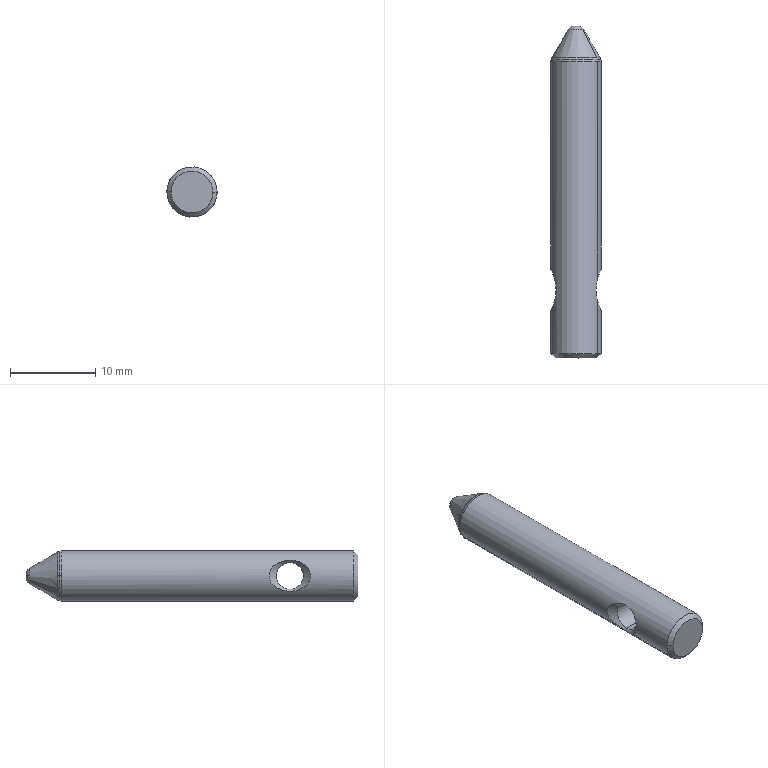Part | NX | features solid 2 | 1 solid | 20 faces | box 5.9 x 39 x 5.9 mm | volume 952.657 mm3 | cone 8 | cylinder 4 | torus 4 | plane 2 | spline 2 | commonest cylinder face diameters 3.2 x2 5.9 x2
STEP:
#1=CARTESIAN_POINT('',(-286.449,2108.126,25.582));
#2=VERTEX_POINT('',#1);
#3=CARTESIAN_POINT('',(-286.869,2108.126,27.147));
#4=VERTEX_POINT('',#3);
#5=CARTESIAN_POINT('',(-283.92,2108.126,27.1));
#6=DIRECTION('',(0.,1.,0.));
#7=DIRECTION('',(-0.8575,0.,-0.5144));
#8=AXIS2_PLACEMENT_3D('',#5,#6,#7);
#9=CIRCLE('',#8,2.95);
#10=EDGE_CURVE('',#2,#4,#9,.T.);
#11=ORIENTED_EDGE('',*,*,#10,.F.);
#12=CARTESIAN_POINT('',(-286.449,2082.541,25.582));
#13=VERTEX_POINT('',#12);
#14=CARTESIAN_POINT('',(-286.449,2108.126,25.582));
#15=DIRECTION('',(-0.000001242,-1.,0.00000207));
#16=VECTOR('',#15,1000.);
#17=LINE('',#14,#16);
#18=EDGE_CURVE('',#13,#2,#17,.F.);
#19=ORIENTED_EDGE('',*,*,#18,.F.);
#20=CARTESIAN_POINT('',(-286.211,2081.278,28.958));
#21=VERTEX_POINT('',#20);
#22=CARTESIAN_POINT('',(-286.211,2081.278,28.958));
#23=CARTESIAN_POINT('',(-286.211,2081.745,28.958));
#24=CARTESIAN_POINT('',(-286.382,2082.647,28.765));
#25=CARTESIAN_POINT('',(-286.775,2083.553,28.042));
#26=CARTESIAN_POINT('',(-286.9,2083.793,27.11));
#27=CARTESIAN_POINT('',(-286.784,2083.508,26.194));
#28=CARTESIAN_POINT('',(-286.562,2082.953,25.77));
#29=CARTESIAN_POINT('',(-286.449,2082.541,25.582));
#30=B_SPLINE_CURVE_WITH_KNOTS('',3,(#22,#23,#24,#25,#26,#27,#28,#29),.UNSPECIFIED.,.F.,.F.,(4,1,1,1,1,4),(0.,0.001381,0.002761,0.003452,0.004142,0.005523),.UNSPECIFIED.);
#31=EDGE_CURVE('',#21,#13,#30,.T.);
#32=ORIENTED_EDGE('',*,*,#31,.F.);
#33=CARTESIAN_POINT('',(-286.449,2080.015,25.582));
#34=VERTEX_POINT('',#33);
#35=CARTESIAN_POINT('',(-286.449,2080.015,25.582));
#36=CARTESIAN_POINT('',(-286.562,2079.603,25.77));
#37=CARTESIAN_POINT('',(-286.782,2079.051,26.189));
#38=CARTESIAN_POINT('',(-286.9,2078.763,27.107));
#39=CARTESIAN_POINT('',(-286.776,2079.,28.039));
#40=CARTESIAN_POINT('',(-286.384,2079.902,28.763));
#41=CARTESIAN_POINT('',(-286.211,2080.811,28.958));
#42=CARTESIAN_POINT('',(-286.211,2081.278,28.958));
#43=B_SPLINE_CURVE_WITH_KNOTS('',3,(#35,#36,#37,#38,#39,#40,#41,#42),.UNSPECIFIED.,.F.,.F.,(4,1,1,1,1,4),(0.,0.001379,0.002068,0.002758,0.004136,0.005515),.UNSPECIFIED.);
#44=EDGE_CURVE('',#34,#21,#43,.T.);
#45=ORIENTED_EDGE('',*,*,#44,.F.);
#46=CARTESIAN_POINT('',(-286.449,2073.778,25.582));
#47=VERTEX_POINT('',#46);
#48=CARTESIAN_POINT('',(-286.449,2080.015,25.582));
#49=DIRECTION('',(0.,-1.,0.));
#50=VECTOR('',#49,1000.);
#51=LINE('',#48,#50);
#52=EDGE_CURVE('',#47,#34,#51,.F.);
#53=ORIENTED_EDGE('',*,*,#52,.F.);
#54=CARTESIAN_POINT('',(-286.869,2073.778,27.147));
#55=VERTEX_POINT('',#54);
#56=CARTESIAN_POINT('',(-283.92,2073.778,27.1));
#57=DIRECTION('',(0.,-1.,0.));
#58=DIRECTION('',(-0.9999,0.,0.01589));
#59=AXIS2_PLACEMENT_3D('',#56,#57,#58);
#60=CIRCLE('',#59,2.95);
#61=EDGE_CURVE('',#55,#47,#60,.T.);
#62=ORIENTED_EDGE('',*,*,#61,.F.);
#63=CARTESIAN_POINT('',(-281.39,2073.778,28.618));
#64=VERTEX_POINT('',#63);
#65=CARTESIAN_POINT('',(-283.92,2073.778,27.1));
#66=DIRECTION('',(0.,-1.,0.));
#67=DIRECTION('',(0.8575,0.,0.5144));
#68=AXIS2_PLACEMENT_3D('',#65,#66,#67);
#69=CIRCLE('',#68,2.95);
#70=EDGE_CURVE('',#64,#55,#69,.T.);
#71=ORIENTED_EDGE('',*,*,#70,.F.);
#72=CARTESIAN_POINT('',(-281.39,2080.015,28.618));
#73=VERTEX_POINT('',#72);
#74=CARTESIAN_POINT('',(-281.39,2080.015,28.618));
#75=DIRECTION('',(0.,-1.,0.));
#76=VECTOR('',#75,1000.);
#77=LINE('',#74,#76);
#78=EDGE_CURVE('',#73,#64,#77,.T.);
#79=ORIENTED_EDGE('',*,*,#78,.F.);
#80=CARTESIAN_POINT('',(-281.57,2081.278,28.884));
#81=VERTEX_POINT('',#80);
#82=CARTESIAN_POINT('',(-281.57,2081.278,28.884));
#83=CARTESIAN_POINT('',(-281.57,2080.836,28.884));
#84=CARTESIAN_POINT('',(-281.496,2080.405,28.795));
#85=CARTESIAN_POINT('',(-281.39,2080.015,28.618));
#86=B_SPLINE_CURVE_WITH_KNOTS('',3,(#82,#83,#84,#85),.UNSPECIFIED.,.F.,.F.,(4,4),(0.,0.001307),.UNSPECIFIED.);
#87=EDGE_CURVE('',#81,#73,#86,.T.);
#88=ORIENTED_EDGE('',*,*,#87,.F.);
#89=CARTESIAN_POINT('',(-281.39,2082.541,28.618));
#90=VERTEX_POINT('',#89);
#91=CARTESIAN_POINT('',(-281.39,2082.541,28.618));
#92=CARTESIAN_POINT('',(-281.497,2082.15,28.795));
#93=CARTESIAN_POINT('',(-281.57,2081.72,28.884));
#94=CARTESIAN_POINT('',(-281.57,2081.278,28.884));
#95=B_SPLINE_CURVE_WITH_KNOTS('',3,(#91,#92,#93,#94),.UNSPECIFIED.,.F.,.F.,(4,4),(0.,0.001307),.UNSPECIFIED.);
#96=EDGE_CURVE('',#90,#81,#95,.T.);
#97=ORIENTED_EDGE('',*,*,#96,.F.);
#98=CARTESIAN_POINT('',(-281.39,2108.126,28.618));
#99=VERTEX_POINT('',#98);
#100=CARTESIAN_POINT('',(-281.39,2108.126,28.618));
#101=DIRECTION('',(0.,-1.,0.));
#102=VECTOR('',#101,1000.);
#103=LINE('',#100,#102);
#104=EDGE_CURVE('',#99,#90,#103,.T.);
#105=ORIENTED_EDGE('',*,*,#104,.F.);
#106=CARTESIAN_POINT('',(-283.92,2108.126,27.1));
#107=DIRECTION('',(0.,1.,0.));
#108=DIRECTION('',(-0.9999,0.,0.01589));
#109=AXIS2_PLACEMENT_3D('',#106,#107,#108);
#110=CIRCLE('',#109,2.95);
#111=EDGE_CURVE('',#4,#99,#110,.T.);
#112=ORIENTED_EDGE('',*,*,#111,.F.);
#113=EDGE_LOOP('',(#11,#19,#32,#45,#53,#62,#71,#79,#88,#97,#105,#112));
#114=FACE_BOUND('',#113,.T.);
#115=CARTESIAN_POINT('',(-283.92,2084.546,27.1));
#116=DIRECTION('',(0.,-1.,0.));
#117=DIRECTION('',(-0.8575,0.,-0.5144));
#118=AXIS2_PLACEMENT_3D('',#115,#116,#117);
#119=CYLINDRICAL_SURFACE('',#118,2.95);
#120=ADVANCED_FACE('',(#114),#119,.T.);
#121=CARTESIAN_POINT('',(-280.97,2108.126,27.053));
#122=VERTEX_POINT('',#121);
#123=CARTESIAN_POINT('',(-283.92,2108.126,27.1));
#124=DIRECTION('',(0.,1.,0.));
#125=DIRECTION('',(0.8575,0.,0.5144));
#126=AXIS2_PLACEMENT_3D('',#123,#124,#125);
#127=CIRCLE('',#126,2.95);
#128=EDGE_CURVE('',#99,#122,#127,.T.);
#129=ORIENTED_EDGE('',*,*,#128,.T.);
#130=CARTESIAN_POINT('',(-280.997,2108.333,27.054));
#131=VERTEX_POINT('',#130);
#132=CARTESIAN_POINT('',(-281.77,2108.126,27.066));
#133=DIRECTION('',(-0.01589,0.,-0.9999));
#134=DIRECTION('',(0.9658,0.2588,-0.01535));
#135=AXIS2_PLACEMENT_3D('',#132,#133,#134);
#136=CIRCLE('',#135,0.8);
#137=EDGE_CURVE('',#122,#131,#136,.F.);
#138=ORIENTED_EDGE('',*,*,#137,.T.);
#139=CARTESIAN_POINT('',(-286.842,2108.333,27.146));
#140=VERTEX_POINT('',#139);
#141=CARTESIAN_POINT('',(-283.92,2108.333,27.1));
#142=DIRECTION('',(0.,-1.,0.));
#143=DIRECTION('',(0.9999,0.,-0.01589));
#144=AXIS2_PLACEMENT_3D('',#141,#142,#143);
#145=CIRCLE('',#144,2.923);
#146=EDGE_CURVE('',#131,#140,#145,.T.);
#147=ORIENTED_EDGE('',*,*,#146,.T.);
#148=CARTESIAN_POINT('',(-286.069,2108.126,27.134));
#149=DIRECTION('',(0.01589,0.,0.9999));
#150=DIRECTION('',(-0.9658,0.2588,0.01535));
#151=AXIS2_PLACEMENT_3D('',#148,#149,#150);
#152=CIRCLE('',#151,0.8);
#153=EDGE_CURVE('',#140,#4,#152,.T.);
#154=ORIENTED_EDGE('',*,*,#153,.T.);
#155=ORIENTED_EDGE('',*,*,#111,.T.);
#156=EDGE_LOOP('',(#129,#138,#147,#154,#155));
#157=FACE_BOUND('',#156,.T.);
#158=CARTESIAN_POINT('',(-283.92,2108.126,27.1));
#159=DIRECTION('',(0.,-1.,0.));
#160=DIRECTION('',(-0.9999,0.,0.01589));
#161=AXIS2_PLACEMENT_3D('',#158,#159,#160);
#162=TOROIDAL_SURFACE('',#161,2.15,0.8);
#163=ADVANCED_FACE('',(#157),#162,.T.);
#164=ORIENTED_EDGE('',*,*,#153,.F.);
#165=CARTESIAN_POINT('',(-283.92,2108.333,27.1));
#166=DIRECTION('',(0.,-1.,0.));
#167=DIRECTION('',(-0.9999,0.,0.01589));
#168=AXIS2_PLACEMENT_3D('',#165,#166,#167);
#169=CIRCLE('',#168,2.923);
#170=EDGE_CURVE('',#140,#131,#169,.T.);
#171=ORIENTED_EDGE('',*,*,#170,.T.);
#172=ORIENTED_EDGE('',*,*,#137,.F.);
#173=CARTESIAN_POINT('',(-283.92,2108.126,27.1));
#174=DIRECTION('',(0.,1.,0.));
#175=DIRECTION('',(0.9999,0.,-0.01589));
#176=AXIS2_PLACEMENT_3D('',#173,#174,#175);
#177=CIRCLE('',#176,2.95);
#178=EDGE_CURVE('',#122,#2,#177,.T.);
#179=ORIENTED_EDGE('',*,*,#178,.T.);
#180=ORIENTED_EDGE('',*,*,#10,.T.);
#181=EDGE_LOOP('',(#164,#171,#172,#179,#180));
#182=FACE_BOUND('',#181,.T.);
#183=CARTESIAN_POINT('',(-283.92,2108.126,27.1));
#184=DIRECTION('',(0.,-1.,0.));
#185=DIRECTION('',(-0.9999,0.,0.01589));
#186=AXIS2_PLACEMENT_3D('',#183,#184,#185);
#187=TOROIDAL_SURFACE('',#186,2.15,0.8);
#188=ADVANCED_FACE('',(#182),#187,.T.);
#189=ORIENTED_EDGE('',*,*,#104,.T.);
#190=CARTESIAN_POINT('',(-281.628,2081.278,25.242));
#191=VERTEX_POINT('',#190);
#192=CARTESIAN_POINT('',(-281.628,2081.278,25.242));
#193=CARTESIAN_POINT('',(-281.628,2081.745,25.242));
#194=CARTESIAN_POINT('',(-281.457,2082.647,25.435));
#195=CARTESIAN_POINT('',(-281.065,2083.553,26.158));
#196=CARTESIAN_POINT('',(-280.94,2083.793,27.09));
#197=CARTESIAN_POINT('',(-281.056,2083.508,28.006));
#198=CARTESIAN_POINT('',(-281.278,2082.953,28.43));
#199=CARTESIAN_POINT('',(-281.39,2082.541,28.618));
#200=B_SPLINE_CURVE_WITH_KNOTS('',3,(#192,#193,#194,#195,#196,#197,#198,#199),.UNSPECIFIED.,.F.,.F.,(4,1,1,1,1,4),(0.,0.001381,0.002761,0.003452,0.004142,0.005523),.UNSPECIFIED.);
#201=EDGE_CURVE('',#191,#90,#200,.T.);
#202=ORIENTED_EDGE('',*,*,#201,.F.);
#203=CARTESIAN_POINT('',(-281.39,2080.015,28.618));
#204=CARTESIAN_POINT('',(-281.278,2079.603,28.43));
#205=CARTESIAN_POINT('',(-281.057,2079.051,28.011));
#206=CARTESIAN_POINT('',(-280.94,2078.763,27.093));
#207=CARTESIAN_POINT('',(-281.063,2079.,26.161));
#208=CARTESIAN_POINT('',(-281.455,2079.902,25.437));
#209=CARTESIAN_POINT('',(-281.628,2080.811,25.242));
#210=CARTESIAN_POINT('',(-281.628,2081.278,25.242));
#211=B_SPLINE_CURVE_WITH_KNOTS('',3,(#203,#204,#205,#206,#207,#208,#209,#210),.UNSPECIFIED.,.F.,.F.,(4,1,1,1,1,4),(0.,0.001379,0.002068,0.002758,0.004136,0.005515),.UNSPECIFIED.);
#212=EDGE_CURVE('',#73,#191,#211,.T.);
#213=ORIENTED_EDGE('',*,*,#212,.F.);
#214=ORIENTED_EDGE('',*,*,#78,.T.);
#215=CARTESIAN_POINT('',(-280.97,2073.778,27.053));
#216=VERTEX_POINT('',#215);
#217=CARTESIAN_POINT('',(-283.92,2073.778,27.1));
#218=DIRECTION('',(0.,-1.,0.));
#219=DIRECTION('',(0.9999,0.,-0.01589));
#220=AXIS2_PLACEMENT_3D('',#217,#218,#219);
#221=CIRCLE('',#220,2.95);
#222=EDGE_CURVE('',#216,#64,#221,.T.);
#223=ORIENTED_EDGE('',*,*,#222,.F.);
#224=CARTESIAN_POINT('',(-283.92,2073.778,27.1));
#225=DIRECTION('',(0.,-1.,0.));
#226=DIRECTION('',(-0.8575,0.,-0.5144));
#227=AXIS2_PLACEMENT_3D('',#224,#225,#226);
#228=CIRCLE('',#227,2.95);
#229=EDGE_CURVE('',#47,#216,#228,.T.);
#230=ORIENTED_EDGE('',*,*,#229,.F.);
#231=ORIENTED_EDGE('',*,*,#52,.T.);
#232=CARTESIAN_POINT('',(-286.269,2081.278,25.316));
#233=VERTEX_POINT('',#232);
#234=CARTESIAN_POINT('',(-286.269,2081.278,25.316));
#235=CARTESIAN_POINT('',(-286.269,2080.836,25.316));
#236=CARTESIAN_POINT('',(-286.343,2080.405,25.405));
#237=CARTESIAN_POINT('',(-286.449,2080.015,25.582));
#238=B_SPLINE_CURVE_WITH_KNOTS('',3,(#234,#235,#236,#237),.UNSPECIFIED.,.F.,.F.,(4,4),(0.,0.001307),.UNSPECIFIED.);
#239=EDGE_CURVE('',#233,#34,#238,.T.);
#240=ORIENTED_EDGE('',*,*,#239,.F.);
#241=CARTESIAN_POINT('',(-286.449,2082.541,25.582));
#242=CARTESIAN_POINT('',(-286.343,2082.15,25.405));
#243=CARTESIAN_POINT('',(-286.269,2081.72,25.316));
#244=CARTESIAN_POINT('',(-286.269,2081.278,25.316));
#245=B_SPLINE_CURVE_WITH_KNOTS('',3,(#241,#242,#243,#244),.UNSPECIFIED.,.F.,.F.,(4,4),(0.,0.001307),.UNSPECIFIED.);
#246=EDGE_CURVE('',#13,#233,#245,.T.);
#247=ORIENTED_EDGE('',*,*,#246,.F.);
#248=ORIENTED_EDGE('',*,*,#18,.T.);
#249=ORIENTED_EDGE('',*,*,#178,.F.);
#250=ORIENTED_EDGE('',*,*,#128,.F.);
#251=EDGE_LOOP('',(#189,#202,#213,#214,#223,#230,#231,#240,#247,#248,#249,#250));
#252=FACE_BOUND('',#251,.T.);
#253=CARTESIAN_POINT('',(-283.92,2084.546,27.1));
#254=DIRECTION('',(0.,-1.,0.));
#255=DIRECTION('',(-0.8575,0.,-0.5144));
#256=AXIS2_PLACEMENT_3D('',#253,#254,#255);
#257=CYLINDRICAL_SURFACE('',#256,2.95);
#258=ADVANCED_FACE('',(#252),#257,.T.);
#259=ORIENTED_EDGE('',*,*,#246,.T.);
#260=CARTESIAN_POINT('',(-286.045,2081.278,25.534));
#261=VERTEX_POINT('',#260);
#262=CARTESIAN_POINT('',(-286.045,2081.278,25.534));
#263=CARTESIAN_POINT('',(-286.12,2081.278,25.461));
#264=CARTESIAN_POINT('',(-286.194,2081.278,25.389));
#265=CARTESIAN_POINT('',(-286.269,2081.278,25.316));
#266=B_SPLINE_CURVE_WITH_KNOTS('',3,(#262,#263,#264,#265),.UNSPECIFIED.,.F.,.F.,(4,4),(0.,0.9996),.UNSPECIFIED.);
#267=EDGE_CURVE('',#261,#233,#266,.T.);
#268=ORIENTED_EDGE('',*,*,#267,.F.);
#269=CARTESIAN_POINT('',(-285.994,2081.278,28.733));
#270=VERTEX_POINT('',#269);
#271=CARTESIAN_POINT('',(-286.019,2081.278,27.133));
#272=DIRECTION('',(0.9999,0.,-0.01589));
#273=DIRECTION('',(-0.01589,0.,-0.9999));
#274=AXIS2_PLACEMENT_3D('',#271,#272,#273);
#275=CIRCLE('',#274,1.6);
#276=EDGE_CURVE('',#261,#270,#275,.T.);
#277=ORIENTED_EDGE('',*,*,#276,.T.);
#278=CARTESIAN_POINT('',(-285.994,2081.278,28.733));
#279=CARTESIAN_POINT('',(-286.066,2081.278,28.808));
#280=CARTESIAN_POINT('',(-286.13,2081.278,28.873));
#281=CARTESIAN_POINT('',(-286.211,2081.278,28.958));
#282=B_SPLINE_CURVE_WITH_KNOTS('',3,(#278,#279,#280,#281),.UNSPECIFIED.,.F.,.F.,(4,4),(0.,0.9999),.UNSPECIFIED.);
#283=EDGE_CURVE('',#21,#270,#282,.F.);
#284=ORIENTED_EDGE('',*,*,#283,.F.);
#285=ORIENTED_EDGE('',*,*,#31,.T.);
#286=EDGE_LOOP('',(#259,#268,#277,#284,#285));
#287=FACE_BOUND('',#286,.T.);
#288=CARTESIAN_POINT('',(-286.445,2081.278,27.14));
#289=DIRECTION('',(-0.9999,0.,0.01589));
#290=DIRECTION('',(0.01589,0.,0.9999));
#291=AXIS2_PLACEMENT_3D('',#288,#289,#290);
#292=CONICAL_SURFACE('',#291,2.026,0.7854);
#293=ADVANCED_FACE('',(#287),#292,.F.);
#294=ORIENTED_EDGE('',*,*,#283,.T.);
#295=CARTESIAN_POINT('',(-286.019,2081.278,27.133));
#296=DIRECTION('',(0.9999,0.,-0.01589));
#297=DIRECTION('',(0.01589,0.,0.9999));
#298=AXIS2_PLACEMENT_3D('',#295,#296,#297);
#299=CIRCLE('',#298,1.6);
#300=EDGE_CURVE('',#270,#261,#299,.T.);
#301=ORIENTED_EDGE('',*,*,#300,.T.);
#302=ORIENTED_EDGE('',*,*,#267,.T.);
#303=ORIENTED_EDGE('',*,*,#239,.T.);
#304=ORIENTED_EDGE('',*,*,#44,.T.);
#305=EDGE_LOOP('',(#294,#301,#302,#303,#304));
#306=FACE_BOUND('',#305,.T.);
#307=CARTESIAN_POINT('',(-286.445,2081.278,27.14));
#308=DIRECTION('',(-0.9999,0.,0.01589));
#309=DIRECTION('',(0.01589,0.,0.9999));
#310=AXIS2_PLACEMENT_3D('',#307,#308,#309);
#311=CONICAL_SURFACE('',#310,2.026,0.7854);
#312=ADVANCED_FACE('',(#306),#311,.F.);
#313=CARTESIAN_POINT('',(-281.845,2081.278,25.467));
#314=VERTEX_POINT('',#313);
#315=CARTESIAN_POINT('',(-281.845,2081.278,25.467));
#316=DIRECTION('',(-0.9999,0.,0.01589));
#317=VECTOR('',#316,1000.);
#318=LINE('',#315,#317);
#319=EDGE_CURVE('',#261,#314,#318,.F.);
#320=ORIENTED_EDGE('',*,*,#319,.F.);
#321=ORIENTED_EDGE('',*,*,#300,.F.);
#322=CARTESIAN_POINT('',(-281.795,2081.278,28.666));
#323=VERTEX_POINT('',#322);
#324=CARTESIAN_POINT('',(-281.795,2081.278,28.666));
#325=DIRECTION('',(-0.9999,0.,0.01589));
#326=VECTOR('',#325,1000.);
#327=LINE('',#324,#326);
#328=EDGE_CURVE('',#323,#270,#327,.T.);
#329=ORIENTED_EDGE('',*,*,#328,.F.);
#330=CARTESIAN_POINT('',(-281.82,2081.278,27.067));
#331=DIRECTION('',(-0.9999,0.,0.01589));
#332=DIRECTION('',(-0.01589,0.,-0.9999));
#333=AXIS2_PLACEMENT_3D('',#330,#331,#332);
#334=CIRCLE('',#333,1.6);
#335=EDGE_CURVE('',#314,#323,#334,.T.);
#336=ORIENTED_EDGE('',*,*,#335,.F.);
#337=EDGE_LOOP('',(#320,#321,#329,#336));
#338=FACE_BOUND('',#337,.T.);
#339=CARTESIAN_POINT('',(-278.92,2081.278,27.021));
#340=DIRECTION('',(-0.9999,0.,0.01589));
#341=DIRECTION('',(0.01589,0.,0.9999));
#342=AXIS2_PLACEMENT_3D('',#339,#340,#341);
#343=CYLINDRICAL_SURFACE('',#342,1.6);
#344=ADVANCED_FACE('',(#338),#343,.F.);
#345=ORIENTED_EDGE('',*,*,#212,.T.);
#346=CARTESIAN_POINT('',(-281.845,2081.278,25.467));
#347=CARTESIAN_POINT('',(-281.773,2081.278,25.392));
#348=CARTESIAN_POINT('',(-281.71,2081.278,25.327));
#349=CARTESIAN_POINT('',(-281.628,2081.278,25.242));
#350=B_SPLINE_CURVE_WITH_KNOTS('',3,(#346,#347,#348,#349),.UNSPECIFIED.,.F.,.F.,(4,4),(0.,0.9999),.UNSPECIFIED.);
#351=EDGE_CURVE('',#191,#314,#350,.F.);
#352=ORIENTED_EDGE('',*,*,#351,.T.);
#353=ORIENTED_EDGE('',*,*,#335,.T.);
#354=CARTESIAN_POINT('',(-281.795,2081.278,28.666));
#355=CARTESIAN_POINT('',(-281.72,2081.278,28.739));
#356=CARTESIAN_POINT('',(-281.645,2081.278,28.811));
#357=CARTESIAN_POINT('',(-281.57,2081.278,28.884));
#358=B_SPLINE_CURVE_WITH_KNOTS('',3,(#354,#355,#356,#357),.UNSPECIFIED.,.F.,.F.,(4,4),(0.,0.9996),.UNSPECIFIED.);
#359=EDGE_CURVE('',#323,#81,#358,.T.);
#360=ORIENTED_EDGE('',*,*,#359,.T.);
#361=ORIENTED_EDGE('',*,*,#87,.T.);
#362=EDGE_LOOP('',(#345,#352,#353,#360,#361));
#363=FACE_BOUND('',#362,.T.);
#364=CARTESIAN_POINT('',(-281.395,2081.278,27.06));
#365=DIRECTION('',(0.9999,0.,-0.01589));
#366=DIRECTION('',(-0.01589,0.,-0.9999));
#367=AXIS2_PLACEMENT_3D('',#364,#365,#366);
#368=CONICAL_SURFACE('',#367,2.026,0.7854);
#369=ADVANCED_FACE('',(#363),#368,.F.);
#370=ORIENTED_EDGE('',*,*,#359,.F.);
#371=CARTESIAN_POINT('',(-281.82,2081.278,27.067));
#372=DIRECTION('',(-0.9999,0.,0.01589));
#373=DIRECTION('',(0.01589,0.,0.9999));
#374=AXIS2_PLACEMENT_3D('',#371,#372,#373);
#375=CIRCLE('',#374,1.6);
#376=EDGE_CURVE('',#323,#314,#375,.T.);
#377=ORIENTED_EDGE('',*,*,#376,.T.);
#378=ORIENTED_EDGE('',*,*,#351,.F.);
#379=ORIENTED_EDGE('',*,*,#201,.T.);
#380=ORIENTED_EDGE('',*,*,#96,.T.);
#381=EDGE_LOOP('',(#370,#377,#378,#379,#380));
#382=FACE_BOUND('',#381,.T.);
#383=CARTESIAN_POINT('',(-281.395,2081.278,27.06));
#384=DIRECTION('',(0.9999,0.,-0.01589));
#385=DIRECTION('',(-0.01589,0.,-0.9999));
#386=AXIS2_PLACEMENT_3D('',#383,#384,#385);
#387=CONICAL_SURFACE('',#386,2.026,0.7854);
#388=ADVANCED_FACE('',(#382),#387,.F.);
#389=ORIENTED_EDGE('',*,*,#328,.T.);
#390=ORIENTED_EDGE('',*,*,#276,.F.);
#391=ORIENTED_EDGE('',*,*,#319,.T.);
#392=ORIENTED_EDGE('',*,*,#376,.F.);
#393=EDGE_LOOP('',(#389,#390,#391,#392));
#394=FACE_BOUND('',#393,.T.);
#395=CARTESIAN_POINT('',(-278.92,2081.278,27.021));
#396=DIRECTION('',(-0.9999,0.,0.01589));
#397=DIRECTION('',(0.01589,0.,0.9999));
#398=AXIS2_PLACEMENT_3D('',#395,#396,#397);
#399=CYLINDRICAL_SURFACE('',#398,1.6);
#400=ADVANCED_FACE('',(#394),#399,.F.);
#401=CARTESIAN_POINT('',(-286.369,2073.278,27.139));
#402=VERTEX_POINT('',#401);
#403=CARTESIAN_POINT('',(-286.369,2073.278,27.139));
#404=DIRECTION('',(-0.707,0.7071,0.01124));
#405=VECTOR('',#404,1000.);
#406=LINE('',#403,#405);
#407=EDGE_CURVE('',#55,#402,#406,.F.);
#408=ORIENTED_EDGE('',*,*,#407,.F.);
#409=ORIENTED_EDGE('',*,*,#61,.T.);
#410=ORIENTED_EDGE('',*,*,#229,.T.);
#411=CARTESIAN_POINT('',(-281.47,2073.278,27.061));
#412=VERTEX_POINT('',#411);
#413=CARTESIAN_POINT('',(-281.47,2073.278,27.061));
#414=DIRECTION('',(0.707,0.7071,-0.01124));
#415=VECTOR('',#414,1000.);
#416=LINE('',#413,#415);
#417=EDGE_CURVE('',#412,#216,#416,.T.);
#418=ORIENTED_EDGE('',*,*,#417,.F.);
#419=CARTESIAN_POINT('',(-283.92,2073.278,27.1));
#420=DIRECTION('',(0.,-1.,0.));
#421=DIRECTION('',(-0.9999,0.,0.01589));
#422=AXIS2_PLACEMENT_3D('',#419,#420,#421);
#423=CIRCLE('',#422,2.45);
#424=EDGE_CURVE('',#402,#412,#423,.T.);
#425=ORIENTED_EDGE('',*,*,#424,.F.);
#426=EDGE_LOOP('',(#408,#409,#410,#418,#425));
#427=FACE_BOUND('',#426,.T.);
#428=CARTESIAN_POINT('',(-283.92,2073.528,27.1));
#429=DIRECTION('',(0.,1.,0.));
#430=DIRECTION('',(0.9999,0.,-0.01589));
#431=AXIS2_PLACEMENT_3D('',#428,#429,#430);
#432=CONICAL_SURFACE('',#431,2.7,0.7854);
#433=ADVANCED_FACE('',(#427),#432,.T.);
#434=ORIENTED_EDGE('',*,*,#424,.T.);
#435=CARTESIAN_POINT('',(-283.92,2073.278,27.1));
#436=DIRECTION('',(0.,-1.,0.));
#437=DIRECTION('',(0.9999,0.,-0.01589));
#438=AXIS2_PLACEMENT_3D('',#435,#436,#437);
#439=CIRCLE('',#438,2.45);
#440=EDGE_CURVE('',#412,#402,#439,.T.);
#441=ORIENTED_EDGE('',*,*,#440,.T.);
#442=EDGE_LOOP('',(#434,#441));
#443=FACE_BOUND('',#442,.T.);
#444=CARTESIAN_POINT('',(-288.503,2073.278,28.246));
#445=DIRECTION('',(0.,-1.,0.));
#446=DIRECTION('',(-0.8575,0.,-0.5144));
#447=AXIS2_PLACEMENT_3D('',#444,#445,#446);
#448=PLANE('',#447);
#449=ADVANCED_FACE('',(#443),#448,.T.);
#450=ORIENTED_EDGE('',*,*,#417,.T.);
#451=ORIENTED_EDGE('',*,*,#222,.T.);
#452=ORIENTED_EDGE('',*,*,#70,.T.);
#453=ORIENTED_EDGE('',*,*,#407,.T.);
#454=ORIENTED_EDGE('',*,*,#440,.F.);
#455=EDGE_LOOP('',(#450,#451,#452,#453,#454));
#456=FACE_BOUND('',#455,.T.);
#457=CARTESIAN_POINT('',(-283.92,2073.528,27.1));
#458=DIRECTION('',(0.,1.,0.));
#459=DIRECTION('',(0.9999,0.,-0.01589));
#460=AXIS2_PLACEMENT_3D('',#457,#458,#459);
#461=CONICAL_SURFACE('',#460,2.7,0.7854);
#462=ADVANCED_FACE('',(#456),#461,.T.);
#463=CARTESIAN_POINT('',(-281.077,2108.526,27.055));
#464=VERTEX_POINT('',#463);
#465=CARTESIAN_POINT('',(-281.77,2108.126,27.066));
#466=DIRECTION('',(-0.01589,0.,-0.9999));
#467=DIRECTION('',(0.8659,0.5,-0.01376));
#468=AXIS2_PLACEMENT_3D('',#465,#466,#467);
#469=CIRCLE('',#468,0.8);
#470=EDGE_CURVE('',#464,#131,#469,.T.);
#471=ORIENTED_EDGE('',*,*,#470,.T.);
#472=ORIENTED_EDGE('',*,*,#170,.F.);
#473=CARTESIAN_POINT('',(-286.762,2108.526,27.145));
#474=VERTEX_POINT('',#473);
#475=CARTESIAN_POINT('',(-286.069,2108.126,27.134));
#476=DIRECTION('',(0.01589,0.,0.9999));
#477=DIRECTION('',(-0.8659,0.5,0.01376));
#478=AXIS2_PLACEMENT_3D('',#475,#476,#477);
#479=CIRCLE('',#478,0.8);
#480=EDGE_CURVE('',#140,#474,#479,.F.);
#481=ORIENTED_EDGE('',*,*,#480,.T.);
#482=CARTESIAN_POINT('',(-286.358,2108.526,25.638));
#483=VERTEX_POINT('',#482);
#484=CARTESIAN_POINT('',(-283.92,2108.526,27.1));
#485=DIRECTION('',(0.,-1.,0.));
#486=DIRECTION('',(-0.9999,0.,0.01589));
#487=AXIS2_PLACEMENT_3D('',#484,#485,#486);
#488=CIRCLE('',#487,2.843);
#489=EDGE_CURVE('',#474,#483,#488,.T.);
#490=ORIENTED_EDGE('',*,*,#489,.T.);
#491=CARTESIAN_POINT('',(-283.92,2108.526,27.1));
#492=DIRECTION('',(0.,-1.,0.));
#493=DIRECTION('',(-0.8575,0.,-0.5144));
#494=AXIS2_PLACEMENT_3D('',#491,#492,#493);
#495=CIRCLE('',#494,2.843);
#496=EDGE_CURVE('',#483,#464,#495,.T.);
#497=ORIENTED_EDGE('',*,*,#496,.T.);
#498=EDGE_LOOP('',(#471,#472,#481,#490,#497));
#499=FACE_BOUND('',#498,.T.);
#500=CARTESIAN_POINT('',(-283.92,2108.126,27.1));
#501=DIRECTION('',(0.,-1.,0.));
#502=DIRECTION('',(-0.9999,0.,0.01589));
#503=AXIS2_PLACEMENT_3D('',#500,#501,#502);
#504=TOROIDAL_SURFACE('',#503,2.15,0.8);
#505=ADVANCED_FACE('',(#499),#504,.T.);
#506=CARTESIAN_POINT('',(-281.482,2108.526,28.562));
#507=VERTEX_POINT('',#506);
#508=CARTESIAN_POINT('',(-283.92,2108.526,27.1));
#509=DIRECTION('',(0.,-1.,0.));
#510=DIRECTION('',(0.9999,0.,-0.01589));
#511=AXIS2_PLACEMENT_3D('',#508,#509,#510);
#512=CIRCLE('',#511,2.843);
#513=EDGE_CURVE('',#464,#507,#512,.T.);
#514=ORIENTED_EDGE('',*,*,#513,.F.);
#515=ORIENTED_EDGE('',*,*,#496,.F.);
#516=CARTESIAN_POINT('',(-284.698,2111.878,26.633));
#517=VERTEX_POINT('',#516);
#518=CARTESIAN_POINT('',(-286.358,2108.526,25.638));
#519=DIRECTION('',(0.4288,0.866,0.2572));
#520=VECTOR('',#519,1000.);
#521=LINE('',#518,#520);
#522=EDGE_CURVE('',#483,#517,#521,.T.);
#523=ORIENTED_EDGE('',*,*,#522,.T.);
#524=CARTESIAN_POINT('',(-283.012,2111.878,27.086));
#525=VERTEX_POINT('',#524);
#526=CARTESIAN_POINT('',(-283.92,2111.878,27.1));
#527=DIRECTION('',(0.,1.,0.));
#528=DIRECTION('',(0.9999,0.,-0.01589));
#529=AXIS2_PLACEMENT_3D('',#526,#527,#528);
#530=CIRCLE('',#529,0.9079);
#531=EDGE_CURVE('',#525,#517,#530,.T.);
#532=ORIENTED_EDGE('',*,*,#531,.F.);
#533=CARTESIAN_POINT('',(-283.141,2111.878,27.567));
#534=VERTEX_POINT('',#533);
#535=CARTESIAN_POINT('',(-283.92,2111.878,27.1));
#536=DIRECTION('',(0.,1.,0.));
#537=DIRECTION('',(0.8575,0.,0.5144));
#538=AXIS2_PLACEMENT_3D('',#535,#536,#537);
#539=CIRCLE('',#538,0.9079);
#540=EDGE_CURVE('',#534,#525,#539,.T.);
#541=ORIENTED_EDGE('',*,*,#540,.F.);
#542=CARTESIAN_POINT('',(-283.141,2111.878,27.567));
#543=DIRECTION('',(0.4288,-0.866,0.2572));
#544=VECTOR('',#543,1000.);
#545=LINE('',#542,#544);
#546=EDGE_CURVE('',#534,#507,#545,.T.);
#547=ORIENTED_EDGE('',*,*,#546,.T.);
#548=EDGE_LOOP('',(#514,#515,#523,#532,#541,#547));
#549=FACE_BOUND('',#548,.T.);
#550=CARTESIAN_POINT('',(-283.92,2110.202,27.1));
#551=DIRECTION('',(0.,-1.,0.));
#552=DIRECTION('',(-0.9999,0.,0.01589));
#553=AXIS2_PLACEMENT_3D('',#550,#551,#552);
#554=CONICAL_SURFACE('',#553,1.875,0.5236);
#555=ADVANCED_FACE('',(#549),#554,.T.);
#556=ORIENTED_EDGE('',*,*,#489,.F.);
#557=CARTESIAN_POINT('',(-283.92,2108.526,27.1));
#558=DIRECTION('',(0.,-1.,0.));
#559=DIRECTION('',(0.8575,0.,0.5144));
#560=AXIS2_PLACEMENT_3D('',#557,#558,#559);
#561=CIRCLE('',#560,2.843);
#562=EDGE_CURVE('',#507,#474,#561,.T.);
#563=ORIENTED_EDGE('',*,*,#562,.F.);
#564=ORIENTED_EDGE('',*,*,#546,.F.);
#565=CARTESIAN_POINT('',(-284.827,2111.878,27.114));
#566=VERTEX_POINT('',#565);
#567=CARTESIAN_POINT('',(-283.92,2111.878,27.1));
#568=DIRECTION('',(0.,1.,0.));
#569=DIRECTION('',(-0.9999,0.,0.01589));
#570=AXIS2_PLACEMENT_3D('',#567,#568,#569);
#571=CIRCLE('',#570,0.9079);
#572=EDGE_CURVE('',#566,#534,#571,.T.);
#573=ORIENTED_EDGE('',*,*,#572,.F.);
#574=CARTESIAN_POINT('',(-283.92,2111.878,27.1));
#575=DIRECTION('',(0.,1.,0.));
#576=DIRECTION('',(-0.8575,0.,-0.5144));
#577=AXIS2_PLACEMENT_3D('',#574,#575,#576);
#578=CIRCLE('',#577,0.9079);
#579=EDGE_CURVE('',#517,#566,#578,.T.);
#580=ORIENTED_EDGE('',*,*,#579,.F.);
#581=ORIENTED_EDGE('',*,*,#522,.F.);
#582=EDGE_LOOP('',(#556,#563,#564,#573,#580,#581));
#583=FACE_BOUND('',#582,.T.);
#584=CARTESIAN_POINT('',(-283.92,2110.202,27.1));
#585=DIRECTION('',(0.,-1.,0.));
#586=DIRECTION('',(-0.9999,0.,0.01589));
#587=AXIS2_PLACEMENT_3D('',#584,#585,#586);
#588=CONICAL_SURFACE('',#587,1.875,0.5236);
#589=ADVANCED_FACE('',(#583),#588,.T.);
#590=CARTESIAN_POINT('',(-283.705,2112.278,27.097));
#591=VERTEX_POINT('',#590);
#592=CARTESIAN_POINT('',(-283.705,2111.478,27.097));
#593=DIRECTION('',(-0.01589,0.,-0.9999));
#594=DIRECTION('',(0.,1.,0.));
#595=AXIS2_PLACEMENT_3D('',#592,#593,#594);
#596=CIRCLE('',#595,0.8);
#597=EDGE_CURVE('',#591,#525,#596,.T.);
#598=ORIENTED_EDGE('',*,*,#597,.T.);
#599=ORIENTED_EDGE('',*,*,#531,.T.);
#600=ORIENTED_EDGE('',*,*,#579,.T.);
#601=CARTESIAN_POINT('',(-284.135,2112.278,27.103));
#602=VERTEX_POINT('',#601);
#603=CARTESIAN_POINT('',(-284.135,2111.478,27.103));
#604=DIRECTION('',(0.01589,0.,0.9999));
#605=DIRECTION('',(0.,1.,0.));
#606=AXIS2_PLACEMENT_3D('',#603,#604,#605);
#607=CIRCLE('',#606,0.8);
#608=EDGE_CURVE('',#566,#602,#607,.F.);
#609=ORIENTED_EDGE('',*,*,#608,.T.);
#610=CARTESIAN_POINT('',(-283.92,2112.278,27.1));
#611=DIRECTION('',(0.,1.,0.));
#612=DIRECTION('',(0.9999,0.,-0.01589));
#613=AXIS2_PLACEMENT_3D('',#610,#611,#612);
#614=CIRCLE('',#613,0.215);
#615=EDGE_CURVE('',#591,#602,#614,.T.);
#616=ORIENTED_EDGE('',*,*,#615,.F.);
#617=EDGE_LOOP('',(#598,#599,#600,#609,#616));
#618=FACE_BOUND('',#617,.T.);
#619=CARTESIAN_POINT('',(-284.082,2112.276,27.14));
#620=CARTESIAN_POINT('',(-284.402,2112.296,27.218));
#621=CARTESIAN_POINT('',(-284.68,2112.131,27.286));
#622=CARTESIAN_POINT('',(-284.824,2111.835,27.321));
#623=CARTESIAN_POINT('',(-284.109,2112.276,27.027));
#624=CARTESIAN_POINT('',(-284.484,2112.296,26.882));
#625=CARTESIAN_POINT('',(-284.81,2112.131,26.757));
#626=CARTESIAN_POINT('',(-284.978,2111.835,26.692));
#627=CARTESIAN_POINT('',(-284.038,2112.276,26.935));
#628=CARTESIAN_POINT('',(-284.273,2112.296,26.609));
#629=CARTESIAN_POINT('',(-284.477,2112.131,26.326));
#630=CARTESIAN_POINT('',(-284.582,2111.835,26.18));
#631=CARTESIAN_POINT('',(-283.922,2112.276,26.933));
#632=CARTESIAN_POINT('',(-283.928,2112.296,26.603));
#633=CARTESIAN_POINT('',(-283.932,2112.131,26.317));
#634=CARTESIAN_POINT('',(-283.935,2111.835,26.169));
#635=CARTESIAN_POINT('',(-283.806,2112.276,26.931));
#636=CARTESIAN_POINT('',(-283.582,2112.296,26.598));
#637=CARTESIAN_POINT('',(-283.388,2112.131,26.308));
#638=CARTESIAN_POINT('',(-283.287,2111.835,26.159));
#639=CARTESIAN_POINT('',(-283.732,2112.276,27.021));
#640=CARTESIAN_POINT('',(-283.362,2112.296,26.865));
#641=CARTESIAN_POINT('',(-283.041,2112.131,26.729));
#642=CARTESIAN_POINT('',(-282.875,2111.835,26.659));
#643=CARTESIAN_POINT('',(-283.756,2112.276,27.134));
#644=CARTESIAN_POINT('',(-283.434,2112.296,27.203));
#645=CARTESIAN_POINT('',(-283.154,2112.131,27.262));
#646=CARTESIAN_POINT('',(-283.009,2111.835,27.292));
#647=(BOUNDED_SURFACE()B_SPLINE_SURFACE(3,3,((#619,#620,#621,#622),(#623,#624,#625,#626),(#627,#628,#629,#630),(#631,#632,#633,#634),(#635,#636,#637,#638),(#639,#640,#641,#642),(#643,#644,#645,#646)),.UNSPECIFIED.,.F.,.F.,.F.)B_SPLINE_SURFACE_WITH_KNOTS((4,3,4),(4,4),(0.,0.5,1.),(0.,1.),.PIECEWISE_BEZIER_KNOTS.)GEOMETRIC_REPRESENTATION_ITEM()RATIONAL_B_SPLINE_SURFACE(((1.343,1.195,1.195,1.343),(1.006,0.895,0.895,1.006),(1.006,0.895,0.895,1.006),(1.343,1.195,1.195,1.343),(1.006,0.895,0.895,1.006),(1.006,0.895,0.895,1.006),(1.343,1.195,1.195,1.343)))REPRESENTATION_ITEM('')SURFACE());
#648=ADVANCED_FACE('',(#618),#647,.T.);
#649=ORIENTED_EDGE('',*,*,#615,.T.);
#650=CARTESIAN_POINT('',(-283.92,2112.278,27.1));
#651=DIRECTION('',(0.,1.,0.));
#652=DIRECTION('',(-0.9999,0.,0.01589));
#653=AXIS2_PLACEMENT_3D('',#650,#651,#652);
#654=CIRCLE('',#653,0.215);
#655=EDGE_CURVE('',#602,#591,#654,.T.);
#656=ORIENTED_EDGE('',*,*,#655,.T.);
#657=EDGE_LOOP('',(#649,#656));
#658=FACE_BOUND('',#657,.T.);
#659=CARTESIAN_POINT('',(-284.366,2112.278,25.316));
#660=DIRECTION('',(0.,1.,0.));
#661=DIRECTION('',(-0.8575,0.,-0.5144));
#662=AXIS2_PLACEMENT_3D('',#659,#660,#661);
#663=PLANE('',#662);
#664=ADVANCED_FACE('',(#658),#663,.T.);
#665=ORIENTED_EDGE('',*,*,#608,.F.);
#666=ORIENTED_EDGE('',*,*,#572,.T.);
#667=ORIENTED_EDGE('',*,*,#540,.T.);
#668=ORIENTED_EDGE('',*,*,#597,.F.);
#669=ORIENTED_EDGE('',*,*,#655,.F.);
#670=EDGE_LOOP('',(#665,#666,#667,#668,#669));
#671=FACE_BOUND('',#670,.T.);
#672=CARTESIAN_POINT('',(-283.758,2112.276,27.06));
#673=CARTESIAN_POINT('',(-283.437,2112.296,26.982));
#674=CARTESIAN_POINT('',(-283.159,2112.131,26.914));
#675=CARTESIAN_POINT('',(-283.016,2111.835,26.879));
#676=CARTESIAN_POINT('',(-283.73,2112.276,27.173));
#677=CARTESIAN_POINT('',(-283.355,2112.296,27.318));
#678=CARTESIAN_POINT('',(-283.03,2112.131,27.443));
#679=CARTESIAN_POINT('',(-282.862,2111.835,27.508));
#680=CARTESIAN_POINT('',(-283.801,2112.276,27.265));
#681=CARTESIAN_POINT('',(-283.566,2112.296,27.591));
#682=CARTESIAN_POINT('',(-283.363,2112.131,27.874));
#683=CARTESIAN_POINT('',(-283.258,2111.835,28.02));
#684=CARTESIAN_POINT('',(-283.917,2112.276,27.267));
#685=CARTESIAN_POINT('',(-283.912,2112.296,27.597));
#686=CARTESIAN_POINT('',(-283.907,2112.131,27.883));
#687=CARTESIAN_POINT('',(-283.905,2111.835,28.031));
#688=CARTESIAN_POINT('',(-284.033,2112.276,27.269));
#689=CARTESIAN_POINT('',(-284.257,2112.296,27.602));
#690=CARTESIAN_POINT('',(-284.452,2112.131,27.892));
#691=CARTESIAN_POINT('',(-284.552,2111.835,28.041));
#692=CARTESIAN_POINT('',(-284.107,2112.276,27.179));
#693=CARTESIAN_POINT('',(-284.477,2112.296,27.335));
#694=CARTESIAN_POINT('',(-284.798,2112.131,27.471));
#695=CARTESIAN_POINT('',(-284.964,2111.835,27.541));
#696=CARTESIAN_POINT('',(-284.083,2112.276,27.066));
#697=CARTESIAN_POINT('',(-284.406,2112.296,26.997));
#698=CARTESIAN_POINT('',(-284.686,2112.131,26.938));
#699=CARTESIAN_POINT('',(-284.83,2111.835,26.908));
#700=(BOUNDED_SURFACE()B_SPLINE_SURFACE(3,3,((#672,#673,#674,#675),(#676,#677,#678,#679),(#680,#681,#682,#683),(#684,#685,#686,#687),(#688,#689,#690,#691),(#692,#693,#694,#695),(#696,#697,#698,#699)),.UNSPECIFIED.,.F.,.F.,.F.)B_SPLINE_SURFACE_WITH_KNOTS((4,3,4),(4,4),(0.,0.5,1.),(0.,1.),.PIECEWISE_BEZIER_KNOTS.)GEOMETRIC_REPRESENTATION_ITEM()RATIONAL_B_SPLINE_SURFACE(((1.343,1.195,1.195,1.343),(1.006,0.895,0.895,1.006),(1.006,0.895,0.895,1.006),(1.343,1.195,1.195,1.343),(1.006,0.895,0.895,1.006),(1.006,0.895,0.895,1.006),(1.343,1.195,1.195,1.343)))REPRESENTATION_ITEM('')SURFACE());
#701=ADVANCED_FACE('',(#671),#700,.T.);
#702=ORIENTED_EDGE('',*,*,#562,.T.);
#703=ORIENTED_EDGE('',*,*,#480,.F.);
#704=ORIENTED_EDGE('',*,*,#146,.F.);
#705=ORIENTED_EDGE('',*,*,#470,.F.);
#706=ORIENTED_EDGE('',*,*,#513,.T.);
#707=EDGE_LOOP('',(#702,#703,#704,#705,#706));
#708=FACE_BOUND('',#707,.T.);
#709=CARTESIAN_POINT('',(-283.92,2108.126,27.1));
#710=DIRECTION('',(0.,-1.,0.));
#711=DIRECTION('',(-0.9999,0.,0.01589));
#712=AXIS2_PLACEMENT_3D('',#709,#710,#711);
#713=TOROIDAL_SURFACE('',#712,2.15,0.8);
#714=ADVANCED_FACE('',(#708),#713,.T.);
#715=CLOSED_SHELL('',(#120,#163,#188,#258,#293,#312,#344,#369,#388,#400,#433,#449,#462,#505,#555,#589,#648,#664,#701,#714));
#716=MANIFOLD_SOLID_BREP('',#715);
#717=(LENGTH_UNIT()NAMED_UNIT(*)SI_UNIT(.MILLI.,.METRE.));
#718=UNCERTAINTY_MEASURE_WITH_UNIT(LENGTH_MEASURE(0.0508),#717,'','');
#719=(NAMED_UNIT(*)PLANE_ANGLE_UNIT()SI_UNIT($,.RADIAN.));
#720=(NAMED_UNIT(*)SI_UNIT($,.STERADIAN.)SOLID_ANGLE_UNIT());
#721=(GEOMETRIC_REPRESENTATION_CONTEXT(3)GLOBAL_UNCERTAINTY_ASSIGNED_CONTEXT((#718))GLOBAL_UNIT_ASSIGNED_CONTEXT((#717,#719,#720))REPRESENTATION_CONTEXT('',''));
#722=ADVANCED_BREP_SHAPE_REPRESENTATION('',(#716),#721);